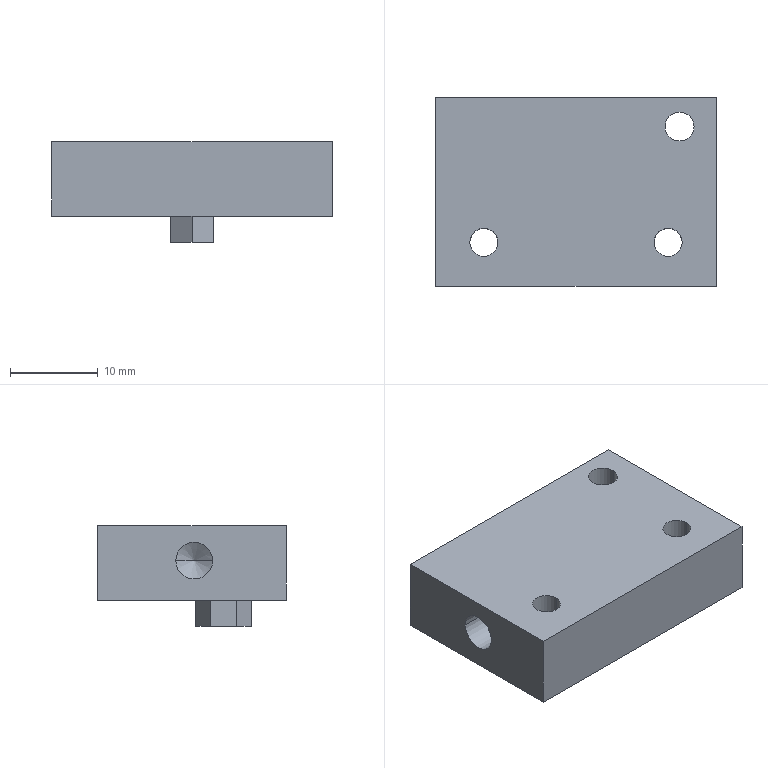Part | NX | 1 solid | 33 faces | box 32 x 21.5 x 11.5 mm | volume 5014 mm3 | plane 18 | cylinder 13 | cone 2 | commonest cylinder face diameters 3.2 x4 6 x4 3.3 x2 4.2 x2 16 x1
STEP:
#1=CARTESIAN_POINT('',(17.,17.5,-162.));
#2=VERTEX_POINT('',#1);
#3=CARTESIAN_POINT('',(25.,9.5,-162.));
#4=VERTEX_POINT('',#3);
#5=CARTESIAN_POINT('',(25.,17.5,-162.));
#6=DIRECTION('',(0.,0.,1.));
#7=DIRECTION('',(1.,0.,0.));
#8=AXIS2_PLACEMENT_3D('',#5,#6,#7);
#9=CIRCLE('',#8,8.);
#10=EDGE_CURVE('',#2,#4,#9,.T.);
#11=ORIENTED_EDGE('',*,*,#10,.T.);
#12=CARTESIAN_POINT('',(29.5,9.5,-162.));
#13=VERTEX_POINT('',#12);
#14=CARTESIAN_POINT('',(0.,9.5,-162.));
#15=DIRECTION('',(1.,0.,0.));
#16=VECTOR('',#15,1000.);
#17=LINE('',#14,#16);
#18=EDGE_CURVE('',#4,#13,#17,.T.);
#19=ORIENTED_EDGE('',*,*,#18,.T.);
#20=CARTESIAN_POINT('',(29.5,-1.,-162.));
#21=VERTEX_POINT('',#20);
#22=CARTESIAN_POINT('',(29.5,0.,-162.));
#23=DIRECTION('',(0.,1.,0.));
#24=VECTOR('',#23,1000.);
#25=LINE('',#22,#24);
#26=EDGE_CURVE('',#21,#13,#25,.T.);
#27=ORIENTED_EDGE('',*,*,#26,.F.);
#28=CARTESIAN_POINT('',(-2.5,-1.,-162.));
#29=VERTEX_POINT('',#28);
#30=CARTESIAN_POINT('',(0.,-1.,-162.));
#31=DIRECTION('',(-1.,0.,0.));
#32=VECTOR('',#31,1000.);
#33=LINE('',#30,#32);
#34=EDGE_CURVE('',#21,#29,#33,.T.);
#35=ORIENTED_EDGE('',*,*,#34,.T.);
#36=CARTESIAN_POINT('',(-2.5,20.5,-162.));
#37=VERTEX_POINT('',#36);
#38=CARTESIAN_POINT('',(-2.5,0.,-162.));
#39=DIRECTION('',(0.,1.,0.));
#40=VECTOR('',#39,1000.);
#41=LINE('',#38,#40);
#42=EDGE_CURVE('',#29,#37,#41,.T.);
#43=ORIENTED_EDGE('',*,*,#42,.T.);
#44=CARTESIAN_POINT('',(17.,20.5,-162.));
#45=VERTEX_POINT('',#44);
#46=CARTESIAN_POINT('',(0.,20.5,-162.));
#47=DIRECTION('',(-1.,0.,0.));
#48=VECTOR('',#47,1000.);
#49=LINE('',#46,#48);
#50=EDGE_CURVE('',#45,#37,#49,.T.);
#51=ORIENTED_EDGE('',*,*,#50,.F.);
#52=CARTESIAN_POINT('',(17.,0.,-162.));
#53=DIRECTION('',(0.,-1.,0.));
#54=VECTOR('',#53,1000.);
#55=LINE('',#52,#54);
#56=EDGE_CURVE('',#45,#2,#55,.T.);
#57=ORIENTED_EDGE('',*,*,#56,.T.);
#58=EDGE_LOOP('',(#11,#19,#27,#35,#43,#51,#57));
#59=FACE_BOUND('',#58,.T.);
#60=CARTESIAN_POINT('',(6.,4.,-162.));
#61=VERTEX_POINT('',#60);
#62=CARTESIAN_POINT('',(0.,4.,-162.));
#63=VERTEX_POINT('',#62);
#64=CARTESIAN_POINT('',(3.,4.,-162.));
#65=DIRECTION('',(0.,0.,1.));
#66=DIRECTION('',(-1.,0.,0.));
#67=AXIS2_PLACEMENT_3D('',#64,#65,#66);
#68=CIRCLE('',#67,3.);
#69=EDGE_CURVE('',#61,#63,#68,.T.);
#70=ORIENTED_EDGE('',*,*,#69,.T.);
#71=CARTESIAN_POINT('',(3.,4.,-162.));
#72=DIRECTION('',(0.,0.,1.));
#73=DIRECTION('',(-1.,0.,0.));
#74=AXIS2_PLACEMENT_3D('',#71,#72,#73);
#75=CIRCLE('',#74,3.);
#76=EDGE_CURVE('',#63,#61,#75,.T.);
#77=ORIENTED_EDGE('',*,*,#76,.T.);
#78=EDGE_LOOP('',(#70,#77));
#79=FACE_BOUND('',#78,.T.);
#80=CARTESIAN_POINT('',(11.,7.658,-162.));
#81=VERTEX_POINT('',#80);
#82=CARTESIAN_POINT('',(11.,4.658,-162.));
#83=VERTEX_POINT('',#82);
#84=CARTESIAN_POINT('',(11.,0.,-162.));
#85=DIRECTION('',(0.,-1.,0.));
#86=VECTOR('',#85,1000.);
#87=LINE('',#84,#86);
#88=EDGE_CURVE('',#81,#83,#87,.T.);
#89=ORIENTED_EDGE('',*,*,#88,.T.);
#90=CARTESIAN_POINT('',(13.5,3.,-162.));
#91=VERTEX_POINT('',#90);
#92=CARTESIAN_POINT('',(0.,11.955,-162.));
#93=DIRECTION('',(0.8333,-0.5528,0.));
#94=VECTOR('',#93,1000.);
#95=LINE('',#92,#94);
#96=EDGE_CURVE('',#83,#91,#95,.T.);
#97=ORIENTED_EDGE('',*,*,#96,.T.);
#98=CARTESIAN_POINT('',(16.,4.658,-162.));
#99=VERTEX_POINT('',#98);
#100=CARTESIAN_POINT('',(0.,-5.955,-162.));
#101=DIRECTION('',(0.8333,0.5528,0.));
#102=VECTOR('',#101,1000.);
#103=LINE('',#100,#102);
#104=EDGE_CURVE('',#91,#99,#103,.T.);
#105=ORIENTED_EDGE('',*,*,#104,.T.);
#106=CARTESIAN_POINT('',(16.,7.658,-162.));
#107=VERTEX_POINT('',#106);
#108=CARTESIAN_POINT('',(16.,0.,-162.));
#109=DIRECTION('',(0.,1.,0.));
#110=VECTOR('',#109,1000.);
#111=LINE('',#108,#110);
#112=EDGE_CURVE('',#99,#107,#111,.T.);
#113=ORIENTED_EDGE('',*,*,#112,.T.);
#114=CARTESIAN_POINT('',(13.5,9.317,-162.));
#115=VERTEX_POINT('',#114);
#116=CARTESIAN_POINT('',(0.,18.272,-162.));
#117=DIRECTION('',(-0.8333,0.5528,0.));
#118=VECTOR('',#117,1000.);
#119=LINE('',#116,#118);
#120=EDGE_CURVE('',#107,#115,#119,.T.);
#121=ORIENTED_EDGE('',*,*,#120,.T.);
#122=CARTESIAN_POINT('',(0.,0.3617,-162.));
#123=DIRECTION('',(-0.8333,-0.5528,0.));
#124=VECTOR('',#123,1000.);
#125=LINE('',#122,#124);
#126=EDGE_CURVE('',#115,#81,#125,.T.);
#127=ORIENTED_EDGE('',*,*,#126,.T.);
#128=EDGE_LOOP('',(#89,#97,#105,#113,#121,#127));
#129=FACE_BOUND('',#128,.T.);
#130=CARTESIAN_POINT('',(27.,4.,-162.));
#131=VERTEX_POINT('',#130);
#132=CARTESIAN_POINT('',(21.,4.,-162.));
#133=VERTEX_POINT('',#132);
#134=CARTESIAN_POINT('',(24.,4.,-162.));
#135=DIRECTION('',(0.,0.,1.));
#136=DIRECTION('',(-1.,0.,0.));
#137=AXIS2_PLACEMENT_3D('',#134,#135,#136);
#138=CIRCLE('',#137,3.);
#139=EDGE_CURVE('',#131,#133,#138,.T.);
#140=ORIENTED_EDGE('',*,*,#139,.T.);
#141=CARTESIAN_POINT('',(24.,4.,-162.));
#142=DIRECTION('',(0.,0.,1.));
#143=DIRECTION('',(-1.,0.,0.));
#144=AXIS2_PLACEMENT_3D('',#141,#142,#143);
#145=CIRCLE('',#144,3.);
#146=EDGE_CURVE('',#133,#131,#145,.T.);
#147=ORIENTED_EDGE('',*,*,#146,.T.);
#148=EDGE_LOOP('',(#140,#147));
#149=FACE_BOUND('',#148,.T.);
#150=CARTESIAN_POINT('',(0.,0.,-162.));
#151=DIRECTION('',(0.,0.,1.));
#152=DIRECTION('',(1.,0.,0.));
#153=AXIS2_PLACEMENT_3D('',#150,#151,#152);
#154=PLANE('',#153);
#155=ADVANCED_FACE('',(#59,#79,#129,#149),#154,.F.);
#156=CARTESIAN_POINT('',(-2.5,-1.,-153.5));
#157=VERTEX_POINT('',#156);
#158=CARTESIAN_POINT('',(-2.5,-1.,0.));
#159=DIRECTION('',(0.,0.,1.));
#160=VECTOR('',#159,1000.);
#161=LINE('',#158,#160);
#162=EDGE_CURVE('',#29,#157,#161,.T.);
#163=ORIENTED_EDGE('',*,*,#162,.F.);
#164=ORIENTED_EDGE('',*,*,#34,.F.);
#165=CARTESIAN_POINT('',(29.5,-1.,-153.5));
#166=VERTEX_POINT('',#165);
#167=CARTESIAN_POINT('',(29.5,-1.,0.));
#168=DIRECTION('',(0.,0.,-1.));
#169=VECTOR('',#168,1000.);
#170=LINE('',#167,#169);
#171=EDGE_CURVE('',#166,#21,#170,.T.);
#172=ORIENTED_EDGE('',*,*,#171,.F.);
#173=CARTESIAN_POINT('',(0.,-1.,-153.5));
#174=DIRECTION('',(1.,0.,0.));
#175=VECTOR('',#174,1000.);
#176=LINE('',#173,#175);
#177=EDGE_CURVE('',#157,#166,#176,.T.);
#178=ORIENTED_EDGE('',*,*,#177,.F.);
#179=EDGE_LOOP('',(#163,#164,#172,#178));
#180=FACE_BOUND('',#179,.T.);
#181=CARTESIAN_POINT('',(0.,-1.,-153.5));
#182=DIRECTION('',(0.,1.,0.));
#183=DIRECTION('',(1.,0.,0.));
#184=AXIS2_PLACEMENT_3D('',#181,#182,#183);
#185=PLANE('',#184);
#186=ADVANCED_FACE('',(#180),#185,.F.);
#187=CARTESIAN_POINT('',(21.,4.,-158.7));
#188=VERTEX_POINT('',#187);
#189=CARTESIAN_POINT('',(27.,4.,-158.7));
#190=VERTEX_POINT('',#189);
#191=CARTESIAN_POINT('',(24.,4.,-158.7));
#192=DIRECTION('',(0.,0.,1.));
#193=DIRECTION('',(-1.,0.,0.));
#194=AXIS2_PLACEMENT_3D('',#191,#192,#193);
#195=CIRCLE('',#194,3.);
#196=EDGE_CURVE('',#188,#190,#195,.T.);
#197=ORIENTED_EDGE('',*,*,#196,.F.);
#198=CARTESIAN_POINT('',(24.,4.,-158.7));
#199=DIRECTION('',(0.,0.,1.));
#200=DIRECTION('',(-1.,0.,0.));
#201=AXIS2_PLACEMENT_3D('',#198,#199,#200);
#202=CIRCLE('',#201,3.);
#203=EDGE_CURVE('',#190,#188,#202,.T.);
#204=ORIENTED_EDGE('',*,*,#203,.F.);
#205=EDGE_LOOP('',(#197,#204));
#206=FACE_BOUND('',#205,.T.);
#207=CARTESIAN_POINT('',(25.6,4.,-158.7));
#208=VERTEX_POINT('',#207);
#209=CARTESIAN_POINT('',(22.4,4.,-158.7));
#210=VERTEX_POINT('',#209);
#211=CARTESIAN_POINT('',(24.,4.,-158.7));
#212=DIRECTION('',(0.,0.,1.));
#213=DIRECTION('',(-1.,0.,0.));
#214=AXIS2_PLACEMENT_3D('',#211,#212,#213);
#215=CIRCLE('',#214,1.6);
#216=EDGE_CURVE('',#208,#210,#215,.T.);
#217=ORIENTED_EDGE('',*,*,#216,.T.);
#218=CARTESIAN_POINT('',(24.,4.,-158.7));
#219=DIRECTION('',(0.,0.,1.));
#220=DIRECTION('',(-1.,0.,0.));
#221=AXIS2_PLACEMENT_3D('',#218,#219,#220);
#222=CIRCLE('',#221,1.6);
#223=EDGE_CURVE('',#210,#208,#222,.T.);
#224=ORIENTED_EDGE('',*,*,#223,.T.);
#225=EDGE_LOOP('',(#217,#224));
#226=FACE_BOUND('',#225,.T.);
#227=CARTESIAN_POINT('',(24.,4.,-158.7));
#228=DIRECTION('',(0.,0.,1.));
#229=DIRECTION('',(1.,0.,0.));
#230=AXIS2_PLACEMENT_3D('',#227,#228,#229);
#231=PLANE('',#230);
#232=ADVANCED_FACE('',(#206,#226),#231,.F.);
#233=CARTESIAN_POINT('',(17.,20.5,-159.));
#234=VERTEX_POINT('',#233);
#235=CARTESIAN_POINT('',(17.,20.5,0.));
#236=DIRECTION('',(0.,0.,-1.));
#237=VECTOR('',#236,1000.);
#238=LINE('',#235,#237);
#239=EDGE_CURVE('',#234,#45,#238,.T.);
#240=ORIENTED_EDGE('',*,*,#239,.T.);
#241=ORIENTED_EDGE('',*,*,#50,.T.);
#242=CARTESIAN_POINT('',(-2.5,20.5,-153.5));
#243=VERTEX_POINT('',#242);
#244=CARTESIAN_POINT('',(-2.5,20.5,0.));
#245=DIRECTION('',(0.,0.,1.));
#246=VECTOR('',#245,1000.);
#247=LINE('',#244,#246);
#248=EDGE_CURVE('',#37,#243,#247,.T.);
#249=ORIENTED_EDGE('',*,*,#248,.T.);
#250=CARTESIAN_POINT('',(29.5,20.5,-153.5));
#251=VERTEX_POINT('',#250);
#252=CARTESIAN_POINT('',(0.,20.5,-153.5));
#253=DIRECTION('',(-1.,0.,0.));
#254=VECTOR('',#253,1000.);
#255=LINE('',#252,#254);
#256=EDGE_CURVE('',#251,#243,#255,.T.);
#257=ORIENTED_EDGE('',*,*,#256,.F.);
#258=CARTESIAN_POINT('',(29.5,20.5,-159.));
#259=VERTEX_POINT('',#258);
#260=CARTESIAN_POINT('',(29.5,20.5,0.));
#261=DIRECTION('',(0.,0.,-1.));
#262=VECTOR('',#261,1000.);
#263=LINE('',#260,#262);
#264=EDGE_CURVE('',#251,#259,#263,.T.);
#265=ORIENTED_EDGE('',*,*,#264,.T.);
#266=CARTESIAN_POINT('',(0.,20.5,-159.));
#267=DIRECTION('',(-1.,0.,0.));
#268=VECTOR('',#267,1000.);
#269=LINE('',#266,#268);
#270=EDGE_CURVE('',#259,#234,#269,.T.);
#271=ORIENTED_EDGE('',*,*,#270,.T.);
#272=EDGE_LOOP('',(#240,#241,#249,#257,#265,#271));
#273=FACE_BOUND('',#272,.T.);
#274=CARTESIAN_POINT('',(27.,20.5,-153.5));
#275=DIRECTION('',(0.,-1.,0.));
#276=DIRECTION('',(0.,0.,-1.));
#277=AXIS2_PLACEMENT_3D('',#274,#275,#276);
#278=PLANE('',#277);
#279=ADVANCED_FACE('',(#273),#278,.F.);
#280=CARTESIAN_POINT('',(25.,9.5,-159.));
#281=VERTEX_POINT('',#280);
#282=CARTESIAN_POINT('',(29.5,9.5,-159.));
#283=VERTEX_POINT('',#282);
#284=CARTESIAN_POINT('',(0.,9.5,-159.));
#285=DIRECTION('',(1.,0.,0.));
#286=VECTOR('',#285,1000.);
#287=LINE('',#284,#286);
#288=EDGE_CURVE('',#281,#283,#287,.T.);
#289=ORIENTED_EDGE('',*,*,#288,.F.);
#290=CARTESIAN_POINT('',(17.,17.5,-159.));
#291=VERTEX_POINT('',#290);
#292=CARTESIAN_POINT('',(25.,17.5,-159.));
#293=DIRECTION('',(0.,0.,1.));
#294=DIRECTION('',(1.,0.,0.));
#295=AXIS2_PLACEMENT_3D('',#292,#293,#294);
#296=CIRCLE('',#295,8.);
#297=EDGE_CURVE('',#291,#281,#296,.T.);
#298=ORIENTED_EDGE('',*,*,#297,.F.);
#299=CARTESIAN_POINT('',(17.,0.,-159.));
#300=DIRECTION('',(0.,-1.,0.));
#301=VECTOR('',#300,1000.);
#302=LINE('',#299,#301);
#303=EDGE_CURVE('',#234,#291,#302,.T.);
#304=ORIENTED_EDGE('',*,*,#303,.F.);
#305=ORIENTED_EDGE('',*,*,#270,.F.);
#306=CARTESIAN_POINT('',(29.5,0.,-159.));
#307=DIRECTION('',(0.,1.,0.));
#308=VECTOR('',#307,1000.);
#309=LINE('',#306,#308);
#310=EDGE_CURVE('',#283,#259,#309,.T.);
#311=ORIENTED_EDGE('',*,*,#310,.F.);
#312=EDGE_LOOP('',(#289,#298,#304,#305,#311));
#313=FACE_BOUND('',#312,.T.);
#314=CARTESIAN_POINT('',(26.95,17.2,-159.));
#315=VERTEX_POINT('',#314);
#316=CARTESIAN_POINT('',(23.65,17.2,-159.));
#317=VERTEX_POINT('',#316);
#318=CARTESIAN_POINT('',(25.3,17.2,-159.));
#319=DIRECTION('',(0.,0.,1.));
#320=DIRECTION('',(1.,0.,0.));
#321=AXIS2_PLACEMENT_3D('',#318,#319,#320);
#322=CIRCLE('',#321,1.65);
#323=EDGE_CURVE('',#315,#317,#322,.T.);
#324=ORIENTED_EDGE('',*,*,#323,.T.);
#325=CARTESIAN_POINT('',(25.3,17.2,-159.));
#326=DIRECTION('',(0.,0.,1.));
#327=DIRECTION('',(1.,0.,0.));
#328=AXIS2_PLACEMENT_3D('',#325,#326,#327);
#329=CIRCLE('',#328,1.65);
#330=EDGE_CURVE('',#317,#315,#329,.T.);
#331=ORIENTED_EDGE('',*,*,#330,.T.);
#332=EDGE_LOOP('',(#324,#331));
#333=FACE_BOUND('',#332,.T.);
#334=CARTESIAN_POINT('',(0.,0.,-159.));
#335=DIRECTION('',(0.,0.,1.));
#336=DIRECTION('',(1.,0.,0.));
#337=AXIS2_PLACEMENT_3D('',#334,#335,#336);
#338=PLANE('',#337);
#339=ADVANCED_FACE('',(#313,#333),#338,.F.);
#340=ORIENTED_EDGE('',*,*,#264,.F.);
#341=CARTESIAN_POINT('',(29.5,0.,-153.5));
#342=DIRECTION('',(0.,1.,0.));
#343=VECTOR('',#342,1000.);
#344=LINE('',#341,#343);
#345=EDGE_CURVE('',#166,#251,#344,.T.);
#346=ORIENTED_EDGE('',*,*,#345,.F.);
#347=ORIENTED_EDGE('',*,*,#171,.T.);
#348=ORIENTED_EDGE('',*,*,#26,.T.);
#349=CARTESIAN_POINT('',(29.5,9.5,0.));
#350=DIRECTION('',(0.,0.,1.));
#351=VECTOR('',#350,1000.);
#352=LINE('',#349,#351);
#353=EDGE_CURVE('',#13,#283,#352,.T.);
#354=ORIENTED_EDGE('',*,*,#353,.T.);
#355=ORIENTED_EDGE('',*,*,#310,.T.);
#356=EDGE_LOOP('',(#340,#346,#347,#348,#354,#355));
#357=FACE_BOUND('',#356,.T.);
#358=CARTESIAN_POINT('',(29.5,0.,-153.5));
#359=DIRECTION('',(-1.,0.,0.));
#360=DIRECTION('',(0.,0.,1.));
#361=AXIS2_PLACEMENT_3D('',#358,#359,#360);
#362=PLANE('',#361);
#363=ADVANCED_FACE('',(#357),#362,.F.);
#364=CARTESIAN_POINT('',(6.,4.,-158.7));
#365=VERTEX_POINT('',#364);
#366=CARTESIAN_POINT('',(0.,4.,-158.7));
#367=VERTEX_POINT('',#366);
#368=CARTESIAN_POINT('',(3.,4.,-158.7));
#369=DIRECTION('',(0.,0.,1.));
#370=DIRECTION('',(-1.,0.,0.));
#371=AXIS2_PLACEMENT_3D('',#368,#369,#370);
#372=CIRCLE('',#371,3.);
#373=EDGE_CURVE('',#365,#367,#372,.T.);
#374=ORIENTED_EDGE('',*,*,#373,.F.);
#375=CARTESIAN_POINT('',(3.,4.,-158.7));
#376=DIRECTION('',(0.,0.,1.));
#377=DIRECTION('',(-1.,0.,0.));
#378=AXIS2_PLACEMENT_3D('',#375,#376,#377);
#379=CIRCLE('',#378,3.);
#380=EDGE_CURVE('',#367,#365,#379,.T.);
#381=ORIENTED_EDGE('',*,*,#380,.F.);
#382=EDGE_LOOP('',(#374,#381));
#383=FACE_BOUND('',#382,.T.);
#384=CARTESIAN_POINT('',(1.4,4.,-158.7));
#385=VERTEX_POINT('',#384);
#386=CARTESIAN_POINT('',(4.6,4.,-158.7));
#387=VERTEX_POINT('',#386);
#388=CARTESIAN_POINT('',(3.,4.,-158.7));
#389=DIRECTION('',(0.,0.,1.));
#390=DIRECTION('',(-1.,0.,0.));
#391=AXIS2_PLACEMENT_3D('',#388,#389,#390);
#392=CIRCLE('',#391,1.6);
#393=EDGE_CURVE('',#385,#387,#392,.T.);
#394=ORIENTED_EDGE('',*,*,#393,.T.);
#395=CARTESIAN_POINT('',(3.,4.,-158.7));
#396=DIRECTION('',(0.,0.,1.));
#397=DIRECTION('',(-1.,0.,0.));
#398=AXIS2_PLACEMENT_3D('',#395,#396,#397);
#399=CIRCLE('',#398,1.6);
#400=EDGE_CURVE('',#387,#385,#399,.T.);
#401=ORIENTED_EDGE('',*,*,#400,.T.);
#402=EDGE_LOOP('',(#394,#401));
#403=FACE_BOUND('',#402,.T.);
#404=CARTESIAN_POINT('',(3.,4.,-158.7));
#405=DIRECTION('',(0.,0.,1.));
#406=DIRECTION('',(1.,0.,0.));
#407=AXIS2_PLACEMENT_3D('',#404,#405,#406);
#408=PLANE('',#407);
#409=ADVANCED_FACE('',(#383,#403),#408,.F.);
#410=ORIENTED_EDGE('',*,*,#239,.F.);
#411=ORIENTED_EDGE('',*,*,#303,.T.);
#412=CARTESIAN_POINT('',(17.,17.5,-162.));
#413=DIRECTION('',(0.,0.,-1.));
#414=VECTOR('',#413,1000.);
#415=LINE('',#412,#414);
#416=EDGE_CURVE('',#291,#2,#415,.T.);
#417=ORIENTED_EDGE('',*,*,#416,.T.);
#418=ORIENTED_EDGE('',*,*,#56,.F.);
#419=EDGE_LOOP('',(#410,#411,#417,#418));
#420=FACE_BOUND('',#419,.T.);
#421=CARTESIAN_POINT('',(17.,19.5,-162.));
#422=DIRECTION('',(1.,0.,0.));
#423=DIRECTION('',(0.,1.,0.));
#424=AXIS2_PLACEMENT_3D('',#421,#422,#423);
#425=PLANE('',#424);
#426=ADVANCED_FACE('',(#420),#425,.T.);
#427=ORIENTED_EDGE('',*,*,#416,.F.);
#428=ORIENTED_EDGE('',*,*,#297,.T.);
#429=CARTESIAN_POINT('',(25.,9.5,-162.));
#430=DIRECTION('',(0.,0.,-1.));
#431=VECTOR('',#430,1000.);
#432=LINE('',#429,#431);
#433=EDGE_CURVE('',#281,#4,#432,.T.);
#434=ORIENTED_EDGE('',*,*,#433,.T.);
#435=ORIENTED_EDGE('',*,*,#10,.F.);
#436=EDGE_LOOP('',(#427,#428,#434,#435));
#437=FACE_BOUND('',#436,.T.);
#438=CARTESIAN_POINT('',(25.,17.5,-162.));
#439=DIRECTION('',(0.,0.,-1.));
#440=DIRECTION('',(1.,0.,0.));
#441=AXIS2_PLACEMENT_3D('',#438,#439,#440);
#442=CYLINDRICAL_SURFACE('',#441,8.);
#443=ADVANCED_FACE('',(#437),#442,.F.);
#444=ORIENTED_EDGE('',*,*,#433,.F.);
#445=ORIENTED_EDGE('',*,*,#288,.T.);
#446=ORIENTED_EDGE('',*,*,#353,.F.);
#447=ORIENTED_EDGE('',*,*,#18,.F.);
#448=EDGE_LOOP('',(#444,#445,#446,#447));
#449=FACE_BOUND('',#448,.T.);
#450=CARTESIAN_POINT('',(27.,9.5,-162.));
#451=DIRECTION('',(0.,1.,0.));
#452=DIRECTION('',(1.,0.,0.));
#453=AXIS2_PLACEMENT_3D('',#450,#451,#452);
#454=PLANE('',#453);
#455=ADVANCED_FACE('',(#449),#454,.T.);
#456=ORIENTED_EDGE('',*,*,#69,.F.);
#457=CARTESIAN_POINT('',(6.,4.,-152.76));
#458=DIRECTION('',(0.,0.,-1.));
#459=VECTOR('',#458,1000.);
#460=LINE('',#457,#459);
#461=EDGE_CURVE('',#61,#365,#460,.F.);
#462=ORIENTED_EDGE('',*,*,#461,.T.);
#463=ORIENTED_EDGE('',*,*,#373,.T.);
#464=CARTESIAN_POINT('',(0.,4.,-152.76));
#465=DIRECTION('',(0.,0.,-1.));
#466=VECTOR('',#465,1000.);
#467=LINE('',#464,#466);
#468=EDGE_CURVE('',#63,#367,#467,.F.);
#469=ORIENTED_EDGE('',*,*,#468,.F.);
#470=EDGE_LOOP('',(#456,#462,#463,#469));
#471=FACE_BOUND('',#470,.T.);
#472=CARTESIAN_POINT('',(3.,4.,-152.76));
#473=DIRECTION('',(0.,0.,-1.));
#474=DIRECTION('',(-1.,0.,0.));
#475=AXIS2_PLACEMENT_3D('',#472,#473,#474);
#476=CYLINDRICAL_SURFACE('',#475,3.);
#477=ADVANCED_FACE('',(#471),#476,.F.);
#478=CARTESIAN_POINT('',(26.95,17.2,-153.5));
#479=VERTEX_POINT('',#478);
#480=CARTESIAN_POINT('',(23.65,17.2,-153.5));
#481=VERTEX_POINT('',#480);
#482=CARTESIAN_POINT('',(25.3,17.2,-153.5));
#483=DIRECTION('',(0.,0.,1.));
#484=DIRECTION('',(1.,0.,0.));
#485=AXIS2_PLACEMENT_3D('',#482,#483,#484);
#486=CIRCLE('',#485,1.65);
#487=EDGE_CURVE('',#479,#481,#486,.T.);
#488=ORIENTED_EDGE('',*,*,#487,.T.);
#489=CARTESIAN_POINT('',(23.65,17.2,-151.045));
#490=DIRECTION('',(0.,0.,-1.));
#491=VECTOR('',#490,1000.);
#492=LINE('',#489,#491);
#493=EDGE_CURVE('',#481,#317,#492,.T.);
#494=ORIENTED_EDGE('',*,*,#493,.T.);
#495=ORIENTED_EDGE('',*,*,#323,.F.);
#496=CARTESIAN_POINT('',(26.95,17.2,-151.045));
#497=DIRECTION('',(0.,0.,-1.));
#498=VECTOR('',#497,1000.);
#499=LINE('',#496,#498);
#500=EDGE_CURVE('',#479,#315,#499,.T.);
#501=ORIENTED_EDGE('',*,*,#500,.F.);
#502=EDGE_LOOP('',(#488,#494,#495,#501));
#503=FACE_BOUND('',#502,.T.);
#504=CARTESIAN_POINT('',(25.3,17.2,-151.045));
#505=DIRECTION('',(0.,0.,-1.));
#506=DIRECTION('',(1.,0.,0.));
#507=AXIS2_PLACEMENT_3D('',#504,#505,#506);
#508=CYLINDRICAL_SURFACE('',#507,1.65);
#509=ADVANCED_FACE('',(#503),#508,.F.);
#510=ORIENTED_EDGE('',*,*,#248,.F.);
#511=ORIENTED_EDGE('',*,*,#42,.F.);
#512=ORIENTED_EDGE('',*,*,#162,.T.);
#513=CARTESIAN_POINT('',(-2.5,0.,-153.5));
#514=DIRECTION('',(0.,-1.,0.));
#515=VECTOR('',#514,1000.);
#516=LINE('',#513,#515);
#517=EDGE_CURVE('',#243,#157,#516,.T.);
#518=ORIENTED_EDGE('',*,*,#517,.F.);
#519=EDGE_LOOP('',(#510,#511,#512,#518));
#520=FACE_BOUND('',#519,.T.);
#521=CARTESIAN_POINT('',(-2.5,11.6,-157.5));
#522=VERTEX_POINT('',#521);
#523=CARTESIAN_POINT('',(-2.5,7.4,-157.5));
#524=VERTEX_POINT('',#523);
#525=CARTESIAN_POINT('',(-2.5,9.5,-157.5));
#526=DIRECTION('',(1.,0.,0.));
#527=DIRECTION('',(0.,1.,0.));
#528=AXIS2_PLACEMENT_3D('',#525,#526,#527);
#529=CIRCLE('',#528,2.1);
#530=EDGE_CURVE('',#522,#524,#529,.T.);
#531=ORIENTED_EDGE('',*,*,#530,.T.);
#532=CARTESIAN_POINT('',(-2.5,9.5,-157.5));
#533=DIRECTION('',(1.,0.,0.));
#534=DIRECTION('',(0.,1.,0.));
#535=AXIS2_PLACEMENT_3D('',#532,#533,#534);
#536=CIRCLE('',#535,2.1);
#537=EDGE_CURVE('',#524,#522,#536,.T.);
#538=ORIENTED_EDGE('',*,*,#537,.T.);
#539=EDGE_LOOP('',(#531,#538));
#540=FACE_BOUND('',#539,.T.);
#541=CARTESIAN_POINT('',(-2.5,19.5,-153.5));
#542=DIRECTION('',(1.,0.,0.));
#543=DIRECTION('',(0.,1.,0.));
#544=AXIS2_PLACEMENT_3D('',#541,#542,#543);
#545=PLANE('',#544);
#546=ADVANCED_FACE('',(#520,#540),#545,.F.);
#547=ORIENTED_EDGE('',*,*,#393,.F.);
#548=CARTESIAN_POINT('',(1.4,4.,-153.5));
#549=VERTEX_POINT('',#548);
#550=CARTESIAN_POINT('',(1.4,4.,-152.26));
#551=DIRECTION('',(0.,0.,-1.));
#552=VECTOR('',#551,1000.);
#553=LINE('',#550,#552);
#554=EDGE_CURVE('',#385,#549,#553,.F.);
#555=ORIENTED_EDGE('',*,*,#554,.T.);
#556=CARTESIAN_POINT('',(4.6,4.,-153.5));
#557=VERTEX_POINT('',#556);
#558=CARTESIAN_POINT('',(3.,4.,-153.5));
#559=DIRECTION('',(0.,0.,1.));
#560=DIRECTION('',(-1.,0.,0.));
#561=AXIS2_PLACEMENT_3D('',#558,#559,#560);
#562=CIRCLE('',#561,1.6);
#563=EDGE_CURVE('',#549,#557,#562,.T.);
#564=ORIENTED_EDGE('',*,*,#563,.T.);
#565=CARTESIAN_POINT('',(4.6,4.,-152.26));
#566=DIRECTION('',(0.,0.,-1.));
#567=VECTOR('',#566,1000.);
#568=LINE('',#565,#567);
#569=EDGE_CURVE('',#387,#557,#568,.F.);
#570=ORIENTED_EDGE('',*,*,#569,.F.);
#571=EDGE_LOOP('',(#547,#555,#564,#570));
#572=FACE_BOUND('',#571,.T.);
#573=CARTESIAN_POINT('',(3.,4.,-152.26));
#574=DIRECTION('',(0.,0.,-1.));
#575=DIRECTION('',(-1.,0.,0.));
#576=AXIS2_PLACEMENT_3D('',#573,#574,#575);
#577=CYLINDRICAL_SURFACE('',#576,1.6);
#578=ADVANCED_FACE('',(#572),#577,.F.);
#579=CARTESIAN_POINT('',(16.,7.658,-165.));
#580=VERTEX_POINT('',#579);
#581=CARTESIAN_POINT('',(13.5,9.317,-165.));
#582=VERTEX_POINT('',#581);
#583=CARTESIAN_POINT('',(0.,18.272,-165.));
#584=DIRECTION('',(-0.8333,0.5528,0.));
#585=VECTOR('',#584,1000.);
#586=LINE('',#583,#585);
#587=EDGE_CURVE('',#580,#582,#586,.T.);
#588=ORIENTED_EDGE('',*,*,#587,.F.);
#589=CARTESIAN_POINT('',(16.,4.658,-165.));
#590=VERTEX_POINT('',#589);
#591=CARTESIAN_POINT('',(16.,0.,-165.));
#592=DIRECTION('',(0.,1.,0.));
#593=VECTOR('',#592,1000.);
#594=LINE('',#591,#593);
#595=EDGE_CURVE('',#590,#580,#594,.T.);
#596=ORIENTED_EDGE('',*,*,#595,.F.);
#597=CARTESIAN_POINT('',(13.5,3.,-165.));
#598=VERTEX_POINT('',#597);
#599=CARTESIAN_POINT('',(0.,-5.955,-165.));
#600=DIRECTION('',(0.8333,0.5528,0.));
#601=VECTOR('',#600,1000.);
#602=LINE('',#599,#601);
#603=EDGE_CURVE('',#598,#590,#602,.T.);
#604=ORIENTED_EDGE('',*,*,#603,.F.);
#605=CARTESIAN_POINT('',(11.,4.658,-165.));
#606=VERTEX_POINT('',#605);
#607=CARTESIAN_POINT('',(0.,11.955,-165.));
#608=DIRECTION('',(-0.8333,0.5528,0.));
#609=VECTOR('',#608,1000.);
#610=LINE('',#607,#609);
#611=EDGE_CURVE('',#598,#606,#610,.T.);
#612=ORIENTED_EDGE('',*,*,#611,.T.);
#613=CARTESIAN_POINT('',(11.,7.658,-165.));
#614=VERTEX_POINT('',#613);
#615=CARTESIAN_POINT('',(11.,0.,-165.));
#616=DIRECTION('',(0.,-1.,0.));
#617=VECTOR('',#616,1000.);
#618=LINE('',#615,#617);
#619=EDGE_CURVE('',#614,#606,#618,.T.);
#620=ORIENTED_EDGE('',*,*,#619,.F.);
#621=CARTESIAN_POINT('',(0.,0.3617,-165.));
#622=DIRECTION('',(-0.8333,-0.5528,0.));
#623=VECTOR('',#622,1000.);
#624=LINE('',#621,#623);
#625=EDGE_CURVE('',#582,#614,#624,.T.);
#626=ORIENTED_EDGE('',*,*,#625,.F.);
#627=EDGE_LOOP('',(#588,#596,#604,#612,#620,#626));
#628=FACE_BOUND('',#627,.T.);
#629=CARTESIAN_POINT('',(0.,0.,-165.));
#630=DIRECTION('',(0.,0.,1.));
#631=DIRECTION('',(1.,0.,0.));
#632=AXIS2_PLACEMENT_3D('',#629,#630,#631);
#633=PLANE('',#632);
#634=ADVANCED_FACE('',(#628),#633,.F.);
#635=ORIENTED_EDGE('',*,*,#139,.F.);
#636=CARTESIAN_POINT('',(27.,4.,-152.76));
#637=DIRECTION('',(0.,0.,-1.));
#638=VECTOR('',#637,1000.);
#639=LINE('',#636,#638);
#640=EDGE_CURVE('',#190,#131,#639,.T.);
#641=ORIENTED_EDGE('',*,*,#640,.F.);
#642=ORIENTED_EDGE('',*,*,#203,.T.);
#643=CARTESIAN_POINT('',(21.,4.,-152.76));
#644=DIRECTION('',(0.,0.,-1.));
#645=VECTOR('',#644,1000.);
#646=LINE('',#643,#645);
#647=EDGE_CURVE('',#188,#133,#646,.T.);
#648=ORIENTED_EDGE('',*,*,#647,.T.);
#649=EDGE_LOOP('',(#635,#641,#642,#648));
#650=FACE_BOUND('',#649,.T.);
#651=CARTESIAN_POINT('',(24.,4.,-152.76));
#652=DIRECTION('',(0.,0.,-1.));
#653=DIRECTION('',(-1.,0.,0.));
#654=AXIS2_PLACEMENT_3D('',#651,#652,#653);
#655=CYLINDRICAL_SURFACE('',#654,3.);
#656=ADVANCED_FACE('',(#650),#655,.F.);
#657=CARTESIAN_POINT('',(12.6,7.4,-157.5));
#658=VERTEX_POINT('',#657);
#659=CARTESIAN_POINT('',(12.6,11.6,-157.5));
#660=VERTEX_POINT('',#659);
#661=CARTESIAN_POINT('',(12.6,9.5,-157.5));
#662=DIRECTION('',(1.,0.,0.));
#663=DIRECTION('',(0.,1.,0.));
#664=AXIS2_PLACEMENT_3D('',#661,#662,#663);
#665=CIRCLE('',#664,2.1);
#666=EDGE_CURVE('',#658,#660,#665,.T.);
#667=ORIENTED_EDGE('',*,*,#666,.T.);
#668=CARTESIAN_POINT('',(14.555,11.6,-157.5));
#669=DIRECTION('',(-1.,0.,0.));
#670=VECTOR('',#669,1000.);
#671=LINE('',#668,#670);
#672=EDGE_CURVE('',#660,#522,#671,.T.);
#673=ORIENTED_EDGE('',*,*,#672,.T.);
#674=ORIENTED_EDGE('',*,*,#537,.F.);
#675=CARTESIAN_POINT('',(14.555,7.4,-157.5));
#676=DIRECTION('',(-1.,0.,0.));
#677=VECTOR('',#676,1000.);
#678=LINE('',#675,#677);
#679=EDGE_CURVE('',#658,#524,#678,.T.);
#680=ORIENTED_EDGE('',*,*,#679,.F.);
#681=EDGE_LOOP('',(#667,#673,#674,#680));
#682=FACE_BOUND('',#681,.T.);
#683=CARTESIAN_POINT('',(14.555,9.5,-157.5));
#684=DIRECTION('',(-1.,0.,0.));
#685=DIRECTION('',(0.,1.,0.));
#686=AXIS2_PLACEMENT_3D('',#683,#684,#685);
#687=CYLINDRICAL_SURFACE('',#686,2.1);
#688=ADVANCED_FACE('',(#682),#687,.F.);
#689=ORIENTED_EDGE('',*,*,#345,.T.);
#690=ORIENTED_EDGE('',*,*,#256,.T.);
#691=ORIENTED_EDGE('',*,*,#517,.T.);
#692=ORIENTED_EDGE('',*,*,#177,.T.);
#693=EDGE_LOOP('',(#689,#690,#691,#692));
#694=FACE_BOUND('',#693,.T.);
#695=CARTESIAN_POINT('',(3.,4.,-153.5));
#696=DIRECTION('',(0.,0.,1.));
#697=DIRECTION('',(-1.,0.,0.));
#698=AXIS2_PLACEMENT_3D('',#695,#696,#697);
#699=CIRCLE('',#698,1.6);
#700=EDGE_CURVE('',#557,#549,#699,.T.);
#701=ORIENTED_EDGE('',*,*,#700,.F.);
#702=ORIENTED_EDGE('',*,*,#563,.F.);
#703=EDGE_LOOP('',(#701,#702));
#704=FACE_BOUND('',#703,.T.);
#705=CARTESIAN_POINT('',(25.6,4.,-153.5));
#706=VERTEX_POINT('',#705);
#707=CARTESIAN_POINT('',(22.4,4.,-153.5));
#708=VERTEX_POINT('',#707);
#709=CARTESIAN_POINT('',(24.,4.,-153.5));
#710=DIRECTION('',(0.,0.,1.));
#711=DIRECTION('',(-1.,0.,0.));
#712=AXIS2_PLACEMENT_3D('',#709,#710,#711);
#713=CIRCLE('',#712,1.6);
#714=EDGE_CURVE('',#706,#708,#713,.T.);
#715=ORIENTED_EDGE('',*,*,#714,.F.);
#716=CARTESIAN_POINT('',(24.,4.,-153.5));
#717=DIRECTION('',(0.,0.,1.));
#718=DIRECTION('',(-1.,0.,0.));
#719=AXIS2_PLACEMENT_3D('',#716,#717,#718);
#720=CIRCLE('',#719,1.6);
#721=EDGE_CURVE('',#708,#706,#720,.T.);
#722=ORIENTED_EDGE('',*,*,#721,.F.);
#723=EDGE_LOOP('',(#715,#722));
#724=FACE_BOUND('',#723,.T.);
#725=ORIENTED_EDGE('',*,*,#487,.F.);
#726=CARTESIAN_POINT('',(25.3,17.2,-153.5));
#727=DIRECTION('',(0.,0.,1.));
#728=DIRECTION('',(1.,0.,0.));
#729=AXIS2_PLACEMENT_3D('',#726,#727,#728);
#730=CIRCLE('',#729,1.65);
#731=EDGE_CURVE('',#481,#479,#730,.T.);
#732=ORIENTED_EDGE('',*,*,#731,.F.);
#733=EDGE_LOOP('',(#725,#732));
#734=FACE_BOUND('',#733,.T.);
#735=CARTESIAN_POINT('',(0.,0.,-153.5));
#736=DIRECTION('',(0.,0.,1.));
#737=DIRECTION('',(1.,0.,0.));
#738=AXIS2_PLACEMENT_3D('',#735,#736,#737);
#739=PLANE('',#738);
#740=ADVANCED_FACE('',(#694,#704,#724,#734),#739,.T.);
#741=ORIENTED_EDGE('',*,*,#714,.T.);
#742=CARTESIAN_POINT('',(22.4,4.,-152.26));
#743=DIRECTION('',(0.,0.,-1.));
#744=VECTOR('',#743,1000.);
#745=LINE('',#742,#744);
#746=EDGE_CURVE('',#210,#708,#745,.F.);
#747=ORIENTED_EDGE('',*,*,#746,.F.);
#748=ORIENTED_EDGE('',*,*,#216,.F.);
#749=CARTESIAN_POINT('',(25.6,4.,-152.26));
#750=DIRECTION('',(0.,0.,-1.));
#751=VECTOR('',#750,1000.);
#752=LINE('',#749,#751);
#753=EDGE_CURVE('',#208,#706,#752,.F.);
#754=ORIENTED_EDGE('',*,*,#753,.T.);
#755=EDGE_LOOP('',(#741,#747,#748,#754));
#756=FACE_BOUND('',#755,.T.);
#757=CARTESIAN_POINT('',(24.,4.,-152.26));
#758=DIRECTION('',(0.,0.,-1.));
#759=DIRECTION('',(-1.,0.,0.));
#760=AXIS2_PLACEMENT_3D('',#757,#758,#759);
#761=CYLINDRICAL_SURFACE('',#760,1.6);
#762=ADVANCED_FACE('',(#756),#761,.F.);
#763=CARTESIAN_POINT('',(13.862,9.5,-157.5));
#764=VERTEX_POINT('',#763);
#765=CARTESIAN_POINT('',(13.218,8.429,-157.5));
#766=DIRECTION('',(-0.515,-0.8572,0.));
#767=VECTOR('',#766,1000.);
#768=LINE('',#765,#767);
#769=EDGE_CURVE('',#658,#764,#768,.F.);
#770=ORIENTED_EDGE('',*,*,#769,.F.);
#771=CARTESIAN_POINT('',(12.6,9.5,-157.5));
#772=DIRECTION('',(1.,0.,0.));
#773=DIRECTION('',(0.,1.,0.));
#774=AXIS2_PLACEMENT_3D('',#771,#772,#773);
#775=CIRCLE('',#774,2.1);
#776=EDGE_CURVE('',#660,#658,#775,.T.);
#777=ORIENTED_EDGE('',*,*,#776,.F.);
#778=CARTESIAN_POINT('',(13.218,10.571,-157.5));
#779=DIRECTION('',(-0.515,0.8572,0.));
#780=VECTOR('',#779,1000.);
#781=LINE('',#778,#780);
#782=EDGE_CURVE('',#660,#764,#781,.F.);
#783=ORIENTED_EDGE('',*,*,#782,.T.);
#784=EDGE_LOOP('',(#770,#777,#783));
#785=FACE_BOUND('',#784,.T.);
#786=CARTESIAN_POINT('',(13.218,9.5,-157.5));
#787=DIRECTION('',(-1.,0.,0.));
#788=DIRECTION('',(0.,1.,0.));
#789=AXIS2_PLACEMENT_3D('',#786,#787,#788);
#790=CONICAL_SURFACE('',#789,1.071,1.03);
#791=ADVANCED_FACE('',(#785),#790,.F.);
#792=CARTESIAN_POINT('',(13.5,9.317,0.));
#793=DIRECTION('',(0.,0.,-1.));
#794=VECTOR('',#793,1000.);
#795=LINE('',#792,#794);
#796=EDGE_CURVE('',#115,#582,#795,.T.);
#797=ORIENTED_EDGE('',*,*,#796,.T.);
#798=ORIENTED_EDGE('',*,*,#625,.T.);
#799=CARTESIAN_POINT('',(11.,7.658,0.));
#800=DIRECTION('',(0.,0.,1.));
#801=VECTOR('',#800,1000.);
#802=LINE('',#799,#801);
#803=EDGE_CURVE('',#614,#81,#802,.T.);
#804=ORIENTED_EDGE('',*,*,#803,.T.);
#805=ORIENTED_EDGE('',*,*,#126,.F.);
#806=EDGE_LOOP('',(#797,#798,#804,#805));
#807=FACE_BOUND('',#806,.T.);
#808=CARTESIAN_POINT('',(13.5,9.317,-162.));
#809=DIRECTION('',(0.5528,-0.8333,0.));
#810=DIRECTION('',(0.,0.,-1.));
#811=AXIS2_PLACEMENT_3D('',#808,#809,#810);
#812=PLANE('',#811);
#813=ADVANCED_FACE('',(#807),#812,.F.);
#814=CARTESIAN_POINT('',(16.,7.658,0.));
#815=DIRECTION('',(0.,0.,1.));
#816=VECTOR('',#815,1000.);
#817=LINE('',#814,#816);
#818=EDGE_CURVE('',#580,#107,#817,.T.);
#819=ORIENTED_EDGE('',*,*,#818,.F.);
#820=ORIENTED_EDGE('',*,*,#587,.T.);
#821=ORIENTED_EDGE('',*,*,#796,.F.);
#822=ORIENTED_EDGE('',*,*,#120,.F.);
#823=EDGE_LOOP('',(#819,#820,#821,#822));
#824=FACE_BOUND('',#823,.T.);
#825=CARTESIAN_POINT('',(16.,7.658,-162.));
#826=DIRECTION('',(-0.5528,-0.8333,0.));
#827=DIRECTION('',(-0.8333,0.5528,0.));
#828=AXIS2_PLACEMENT_3D('',#825,#826,#827);
#829=PLANE('',#828);
#830=ADVANCED_FACE('',(#824),#829,.F.);
#831=CARTESIAN_POINT('',(16.,4.658,0.));
#832=DIRECTION('',(0.,0.,-1.));
#833=VECTOR('',#832,1000.);
#834=LINE('',#831,#833);
#835=EDGE_CURVE('',#99,#590,#834,.T.);
#836=ORIENTED_EDGE('',*,*,#835,.T.);
#837=ORIENTED_EDGE('',*,*,#595,.T.);
#838=ORIENTED_EDGE('',*,*,#818,.T.);
#839=ORIENTED_EDGE('',*,*,#112,.F.);
#840=EDGE_LOOP('',(#836,#837,#838,#839));
#841=FACE_BOUND('',#840,.T.);
#842=CARTESIAN_POINT('',(16.,4.658,-162.));
#843=DIRECTION('',(-1.,0.,0.));
#844=DIRECTION('',(0.,0.,1.));
#845=AXIS2_PLACEMENT_3D('',#842,#843,#844);
#846=PLANE('',#845);
#847=ADVANCED_FACE('',(#841),#846,.F.);
#848=CARTESIAN_POINT('',(13.5,3.,0.));
#849=DIRECTION('',(0.,0.,-1.));
#850=VECTOR('',#849,1000.);
#851=LINE('',#848,#850);
#852=EDGE_CURVE('',#91,#598,#851,.T.);
#853=ORIENTED_EDGE('',*,*,#852,.T.);
#854=ORIENTED_EDGE('',*,*,#603,.T.);
#855=ORIENTED_EDGE('',*,*,#835,.F.);
#856=ORIENTED_EDGE('',*,*,#104,.F.);
#857=EDGE_LOOP('',(#853,#854,#855,#856));
#858=FACE_BOUND('',#857,.T.);
#859=CARTESIAN_POINT('',(13.5,3.,-162.));
#860=DIRECTION('',(-0.5528,0.8333,0.));
#861=DIRECTION('',(0.,0.,1.));
#862=AXIS2_PLACEMENT_3D('',#859,#860,#861);
#863=PLANE('',#862);
#864=ADVANCED_FACE('',(#858),#863,.F.);
#865=CARTESIAN_POINT('',(11.,4.658,0.));
#866=DIRECTION('',(0.,0.,1.));
#867=VECTOR('',#866,1000.);
#868=LINE('',#865,#867);
#869=EDGE_CURVE('',#606,#83,#868,.T.);
#870=ORIENTED_EDGE('',*,*,#869,.F.);
#871=ORIENTED_EDGE('',*,*,#611,.F.);
#872=ORIENTED_EDGE('',*,*,#852,.F.);
#873=ORIENTED_EDGE('',*,*,#96,.F.);
#874=EDGE_LOOP('',(#870,#871,#872,#873));
#875=FACE_BOUND('',#874,.T.);
#876=CARTESIAN_POINT('',(11.,4.658,-162.));
#877=DIRECTION('',(0.5528,0.8333,0.));
#878=DIRECTION('',(0.,0.,-1.));
#879=AXIS2_PLACEMENT_3D('',#876,#877,#878);
#880=PLANE('',#879);
#881=ADVANCED_FACE('',(#875),#880,.F.);
#882=ORIENTED_EDGE('',*,*,#803,.F.);
#883=ORIENTED_EDGE('',*,*,#619,.T.);
#884=ORIENTED_EDGE('',*,*,#869,.T.);
#885=ORIENTED_EDGE('',*,*,#88,.F.);
#886=EDGE_LOOP('',(#882,#883,#884,#885));
#887=FACE_BOUND('',#886,.T.);
#888=CARTESIAN_POINT('',(11.,7.658,-162.));
#889=DIRECTION('',(1.,0.,0.));
#890=DIRECTION('',(0.,1.,0.));
#891=AXIS2_PLACEMENT_3D('',#888,#889,#890);
#892=PLANE('',#891);
#893=ADVANCED_FACE('',(#887),#892,.F.);
#894=ORIENTED_EDGE('',*,*,#196,.T.);
#895=ORIENTED_EDGE('',*,*,#640,.T.);
#896=ORIENTED_EDGE('',*,*,#146,.F.);
#897=ORIENTED_EDGE('',*,*,#647,.F.);
#898=EDGE_LOOP('',(#894,#895,#896,#897));
#899=FACE_BOUND('',#898,.T.);
#900=CARTESIAN_POINT('',(24.,4.,-152.76));
#901=DIRECTION('',(0.,0.,-1.));
#902=DIRECTION('',(-1.,0.,0.));
#903=AXIS2_PLACEMENT_3D('',#900,#901,#902);
#904=CYLINDRICAL_SURFACE('',#903,3.);
#905=ADVANCED_FACE('',(#899),#904,.F.);
#906=ORIENTED_EDGE('',*,*,#468,.T.);
#907=ORIENTED_EDGE('',*,*,#380,.T.);
#908=ORIENTED_EDGE('',*,*,#461,.F.);
#909=ORIENTED_EDGE('',*,*,#76,.F.);
#910=EDGE_LOOP('',(#906,#907,#908,#909));
#911=FACE_BOUND('',#910,.T.);
#912=CARTESIAN_POINT('',(3.,4.,-152.76));
#913=DIRECTION('',(0.,0.,-1.));
#914=DIRECTION('',(-1.,0.,0.));
#915=AXIS2_PLACEMENT_3D('',#912,#913,#914);
#916=CYLINDRICAL_SURFACE('',#915,3.);
#917=ADVANCED_FACE('',(#911),#916,.F.);
#918=ORIENTED_EDGE('',*,*,#500,.T.);
#919=ORIENTED_EDGE('',*,*,#330,.F.);
#920=ORIENTED_EDGE('',*,*,#493,.F.);
#921=ORIENTED_EDGE('',*,*,#731,.T.);
#922=EDGE_LOOP('',(#918,#919,#920,#921));
#923=FACE_BOUND('',#922,.T.);
#924=CARTESIAN_POINT('',(25.3,17.2,-151.045));
#925=DIRECTION('',(0.,0.,-1.));
#926=DIRECTION('',(1.,0.,0.));
#927=AXIS2_PLACEMENT_3D('',#924,#925,#926);
#928=CYLINDRICAL_SURFACE('',#927,1.65);
#929=ADVANCED_FACE('',(#923),#928,.F.);
#930=ORIENTED_EDGE('',*,*,#746,.T.);
#931=ORIENTED_EDGE('',*,*,#721,.T.);
#932=ORIENTED_EDGE('',*,*,#753,.F.);
#933=ORIENTED_EDGE('',*,*,#223,.F.);
#934=EDGE_LOOP('',(#930,#931,#932,#933));
#935=FACE_BOUND('',#934,.T.);
#936=CARTESIAN_POINT('',(24.,4.,-152.26));
#937=DIRECTION('',(0.,0.,-1.));
#938=DIRECTION('',(-1.,0.,0.));
#939=AXIS2_PLACEMENT_3D('',#936,#937,#938);
#940=CYLINDRICAL_SURFACE('',#939,1.6);
#941=ADVANCED_FACE('',(#935),#940,.F.);
#942=ORIENTED_EDGE('',*,*,#700,.T.);
#943=ORIENTED_EDGE('',*,*,#554,.F.);
#944=ORIENTED_EDGE('',*,*,#400,.F.);
#945=ORIENTED_EDGE('',*,*,#569,.T.);
#946=EDGE_LOOP('',(#942,#943,#944,#945));
#947=FACE_BOUND('',#946,.T.);
#948=CARTESIAN_POINT('',(3.,4.,-152.26));
#949=DIRECTION('',(0.,0.,-1.));
#950=DIRECTION('',(-1.,0.,0.));
#951=AXIS2_PLACEMENT_3D('',#948,#949,#950);
#952=CYLINDRICAL_SURFACE('',#951,1.6);
#953=ADVANCED_FACE('',(#947),#952,.F.);
#954=ORIENTED_EDGE('',*,*,#530,.F.);
#955=ORIENTED_EDGE('',*,*,#672,.F.);
#956=ORIENTED_EDGE('',*,*,#776,.T.);
#957=ORIENTED_EDGE('',*,*,#679,.T.);
#958=EDGE_LOOP('',(#954,#955,#956,#957));
#959=FACE_BOUND('',#958,.T.);
#960=CARTESIAN_POINT('',(14.555,9.5,-157.5));
#961=DIRECTION('',(-1.,0.,0.));
#962=DIRECTION('',(0.,1.,0.));
#963=AXIS2_PLACEMENT_3D('',#960,#961,#962);
#964=CYLINDRICAL_SURFACE('',#963,2.1);
#965=ADVANCED_FACE('',(#959),#964,.F.);
#966=ORIENTED_EDGE('',*,*,#666,.F.);
#967=ORIENTED_EDGE('',*,*,#769,.T.);
#968=ORIENTED_EDGE('',*,*,#782,.F.);
#969=EDGE_LOOP('',(#966,#967,#968));
#970=FACE_BOUND('',#969,.T.);
#971=CARTESIAN_POINT('',(13.218,9.5,-157.5));
#972=DIRECTION('',(-1.,0.,0.));
#973=DIRECTION('',(0.,1.,0.));
#974=AXIS2_PLACEMENT_3D('',#971,#972,#973);
#975=CONICAL_SURFACE('',#974,1.071,1.03);
#976=ADVANCED_FACE('',(#970),#975,.F.);
#977=CLOSED_SHELL('',(#155,#186,#232,#279,#339,#363,#409,#426,#443,#455,#477,#509,#546,#578,#634,#656,#688,#740,#762,#791,#813,#830,#847,#864,#881,#893,#905,#917,#929,#941,#953,#965,#976));
#978=MANIFOLD_SOLID_BREP('',#977);
#979=(LENGTH_UNIT()NAMED_UNIT(*)SI_UNIT(.MILLI.,.METRE.));
#980=UNCERTAINTY_MEASURE_WITH_UNIT(LENGTH_MEASURE(0.00001),#979,'','');
#981=(NAMED_UNIT(*)PLANE_ANGLE_UNIT()SI_UNIT($,.RADIAN.));
#982=(NAMED_UNIT(*)SI_UNIT($,.STERADIAN.)SOLID_ANGLE_UNIT());
#983=(GEOMETRIC_REPRESENTATION_CONTEXT(3)GLOBAL_UNCERTAINTY_ASSIGNED_CONTEXT((#980))GLOBAL_UNIT_ASSIGNED_CONTEXT((#979,#981,#982))REPRESENTATION_CONTEXT('',''));
#984=ADVANCED_BREP_SHAPE_REPRESENTATION('',(#978),#983);